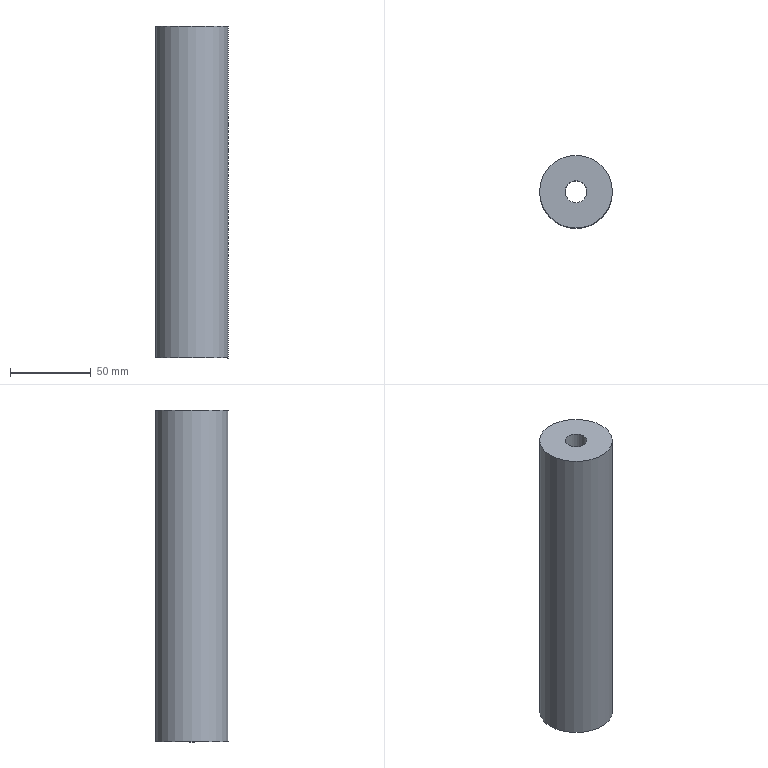Part | NX | features solid 2 | 1 solid | 6 faces | box 45 x 45 x 205.001 mm | volume 288965 mm3 | plane 3 | cylinder 3 | commonest cylinder face diameters 13.507 x1 20.008 x1 45 x1
STEP:
#1=CARTESIAN_POINT('',(-415.019,101.595,-13.871));
#2=VERTEX_POINT('',#1);
#3=CARTESIAN_POINT('',(-425.023,101.595,-13.871));
#4=DIRECTION('',(0.,0.,1.));
#5=DIRECTION('',(1.,0.,0.));
#6=AXIS2_PLACEMENT_3D('',#3,#4,#5);
#7=CIRCLE('',#6,10.004);
#8=EDGE_CURVE('',#2,#2,#7,.T.);
#9=ORIENTED_EDGE('',*,*,#8,.T.);
#10=EDGE_LOOP('',(#9));
#11=FACE_BOUND('',#10,.T.);
#12=CARTESIAN_POINT('',(-402.523,101.595,-13.871));
#13=VERTEX_POINT('',#12);
#14=CARTESIAN_POINT('',(-425.023,101.595,-13.871));
#15=DIRECTION('',(0.,0.,-1.));
#16=DIRECTION('',(1.,0.,0.));
#17=AXIS2_PLACEMENT_3D('',#14,#15,#16);
#18=CIRCLE('',#17,22.5);
#19=EDGE_CURVE('',#13,#13,#18,.T.);
#20=ORIENTED_EDGE('',*,*,#19,.T.);
#21=EDGE_LOOP('',(#20));
#22=FACE_BOUND('',#21,.T.);
#23=CARTESIAN_POINT('',(-1025.023,91.595,-13.871));
#24=DIRECTION('',(0.,0.,-1.));
#25=DIRECTION('',(0.,1.,0.));
#26=AXIS2_PLACEMENT_3D('',#23,#24,#25);
#27=PLANE('',#26);
#28=ADVANCED_FACE('',(#11,#22),#27,.T.);
#29=ORIENTED_EDGE('',*,*,#19,.F.);
#30=EDGE_LOOP('',(#29));
#31=FACE_BOUND('',#30,.T.);
#32=CARTESIAN_POINT('',(-402.523,101.595,191.13));
#33=VERTEX_POINT('',#32);
#34=CARTESIAN_POINT('',(-425.023,101.595,191.13));
#35=DIRECTION('',(0.,0.,-1.));
#36=DIRECTION('',(1.,0.,0.));
#37=AXIS2_PLACEMENT_3D('',#34,#35,#36);
#38=CIRCLE('',#37,22.5);
#39=EDGE_CURVE('',#33,#33,#38,.T.);
#40=ORIENTED_EDGE('',*,*,#39,.T.);
#41=EDGE_LOOP('',(#40));
#42=FACE_BOUND('',#41,.T.);
#43=CARTESIAN_POINT('',(-425.023,101.595,-39.121));
#44=DIRECTION('',(0.,0.,-1.));
#45=DIRECTION('',(0.,1.,0.));
#46=AXIS2_PLACEMENT_3D('',#43,#44,#45);
#47=CYLINDRICAL_SURFACE('',#46,22.5);
#48=ADVANCED_FACE('',(#31,#42),#47,.T.);
#49=CARTESIAN_POINT('',(-418.27,101.595,191.13));
#50=VERTEX_POINT('',#49);
#51=CARTESIAN_POINT('',(-425.023,101.595,191.13));
#52=DIRECTION('',(0.,0.,-1.));
#53=DIRECTION('',(1.,0.,0.));
#54=AXIS2_PLACEMENT_3D('',#51,#52,#53);
#55=CIRCLE('',#54,6.753);
#56=EDGE_CURVE('',#50,#50,#55,.T.);
#57=ORIENTED_EDGE('',*,*,#56,.T.);
#58=EDGE_LOOP('',(#57));
#59=FACE_BOUND('',#58,.T.);
#60=ORIENTED_EDGE('',*,*,#39,.F.);
#61=EDGE_LOOP('',(#60));
#62=FACE_BOUND('',#61,.T.);
#63=CARTESIAN_POINT('',(3549.955,-125.809,191.13));
#64=DIRECTION('',(0.,0.,-1.));
#65=DIRECTION('',(1.,0.,0.));
#66=AXIS2_PLACEMENT_3D('',#63,#64,#65);
#67=PLANE('',#66);
#68=ADVANCED_FACE('',(#59,#62),#67,.F.);
#69=ORIENTED_EDGE('',*,*,#8,.F.);
#70=EDGE_LOOP('',(#69));
#71=FACE_BOUND('',#70,.T.);
#72=CARTESIAN_POINT('',(-415.019,101.595,31.129));
#73=VERTEX_POINT('',#72);
#74=CARTESIAN_POINT('',(-425.023,101.595,31.129));
#75=DIRECTION('',(0.,0.,-1.));
#76=DIRECTION('',(1.,0.,0.));
#77=AXIS2_PLACEMENT_3D('',#74,#75,#76);
#78=CIRCLE('',#77,10.004);
#79=EDGE_CURVE('',#73,#73,#78,.F.);
#80=ORIENTED_EDGE('',*,*,#79,.T.);
#81=EDGE_LOOP('',(#80));
#82=FACE_BOUND('',#81,.T.);
#83=CARTESIAN_POINT('',(-425.023,101.595,-13.871));
#84=DIRECTION('',(0.,0.,1.));
#85=DIRECTION('',(1.,0.,0.));
#86=AXIS2_PLACEMENT_3D('',#83,#84,#85);
#87=CYLINDRICAL_SURFACE('',#86,10.004);
#88=ADVANCED_FACE('',(#71,#82),#87,.F.);
#89=CARTESIAN_POINT('',(-431.777,101.595,31.129));
#90=VERTEX_POINT('',#89);
#91=CARTESIAN_POINT('',(-425.023,101.595,31.129));
#92=DIRECTION('',(0.,0.,1.));
#93=DIRECTION('',(-1.,0.,0.));
#94=AXIS2_PLACEMENT_3D('',#91,#92,#93);
#95=CIRCLE('',#94,6.753);
#96=EDGE_CURVE('',#90,#90,#95,.T.);
#97=ORIENTED_EDGE('',*,*,#96,.F.);
#98=EDGE_LOOP('',(#97));
#99=FACE_BOUND('',#98,.T.);
#100=ORIENTED_EDGE('',*,*,#56,.F.);
#101=EDGE_LOOP('',(#100));
#102=FACE_BOUND('',#101,.T.);
#103=CARTESIAN_POINT('',(-425.023,101.595,-73.871));
#104=DIRECTION('',(0.,0.,1.));
#105=DIRECTION('',(1.,0.,0.));
#106=AXIS2_PLACEMENT_3D('',#103,#104,#105);
#107=CYLINDRICAL_SURFACE('',#106,6.753);
#108=ADVANCED_FACE('',(#99,#102),#107,.F.);
#109=ORIENTED_EDGE('',*,*,#96,.T.);
#110=EDGE_LOOP('',(#109));
#111=FACE_BOUND('',#110,.T.);
#112=ORIENTED_EDGE('',*,*,#79,.F.);
#113=EDGE_LOOP('',(#112));
#114=FACE_BOUND('',#113,.T.);
#115=CARTESIAN_POINT('',(-425.023,101.595,31.129));
#116=DIRECTION('',(0.,0.,1.));
#117=DIRECTION('',(-1.,0.,0.));
#118=AXIS2_PLACEMENT_3D('',#115,#116,#117);
#119=PLANE('',#118);
#120=ADVANCED_FACE('',(#111,#114),#119,.F.);
#121=CLOSED_SHELL('',(#28,#48,#68,#88,#108,#120));
#122=MANIFOLD_SOLID_BREP('',#121);
#123=(LENGTH_UNIT()NAMED_UNIT(*)SI_UNIT(.MILLI.,.METRE.));
#124=UNCERTAINTY_MEASURE_WITH_UNIT(LENGTH_MEASURE(0.00001),#123,'','');
#125=(NAMED_UNIT(*)PLANE_ANGLE_UNIT()SI_UNIT($,.RADIAN.));
#126=(NAMED_UNIT(*)SI_UNIT($,.STERADIAN.)SOLID_ANGLE_UNIT());
#127=(GEOMETRIC_REPRESENTATION_CONTEXT(3)GLOBAL_UNCERTAINTY_ASSIGNED_CONTEXT((#124))GLOBAL_UNIT_ASSIGNED_CONTEXT((#123,#125,#126))REPRESENTATION_CONTEXT('',''));
#128=ADVANCED_BREP_SHAPE_REPRESENTATION('',(#122),#127);